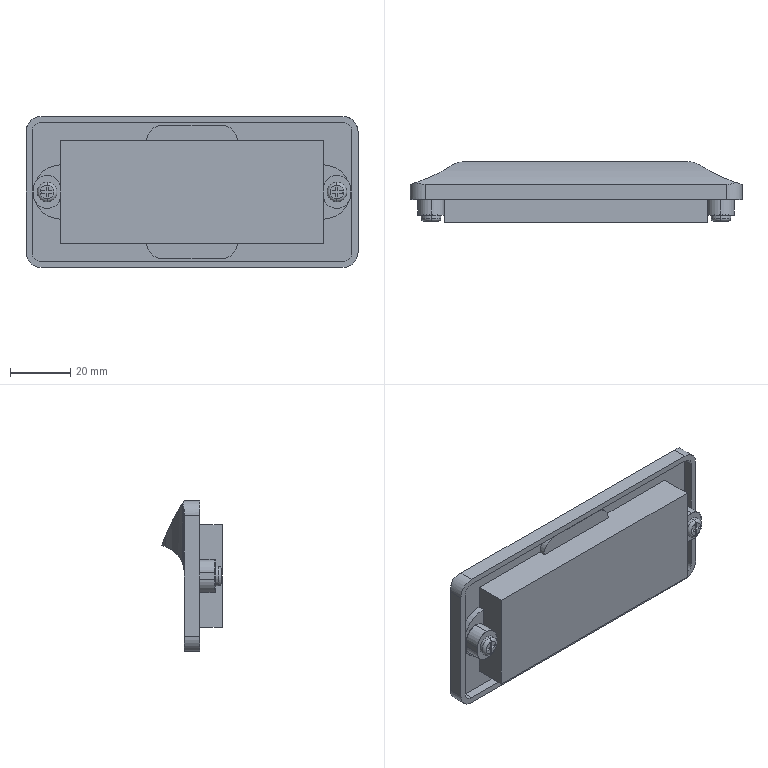Part | NX | features BREP 1 | 1 solid | 139 faces | box 110 x 20 x 50 mm | volume 29039 mm3 | plane 73 | cylinder 62 | torus 4 | commonest cylinder face diameters 6 x8 10 x8 8.6 x6 9 x6 4 x4 5 x4